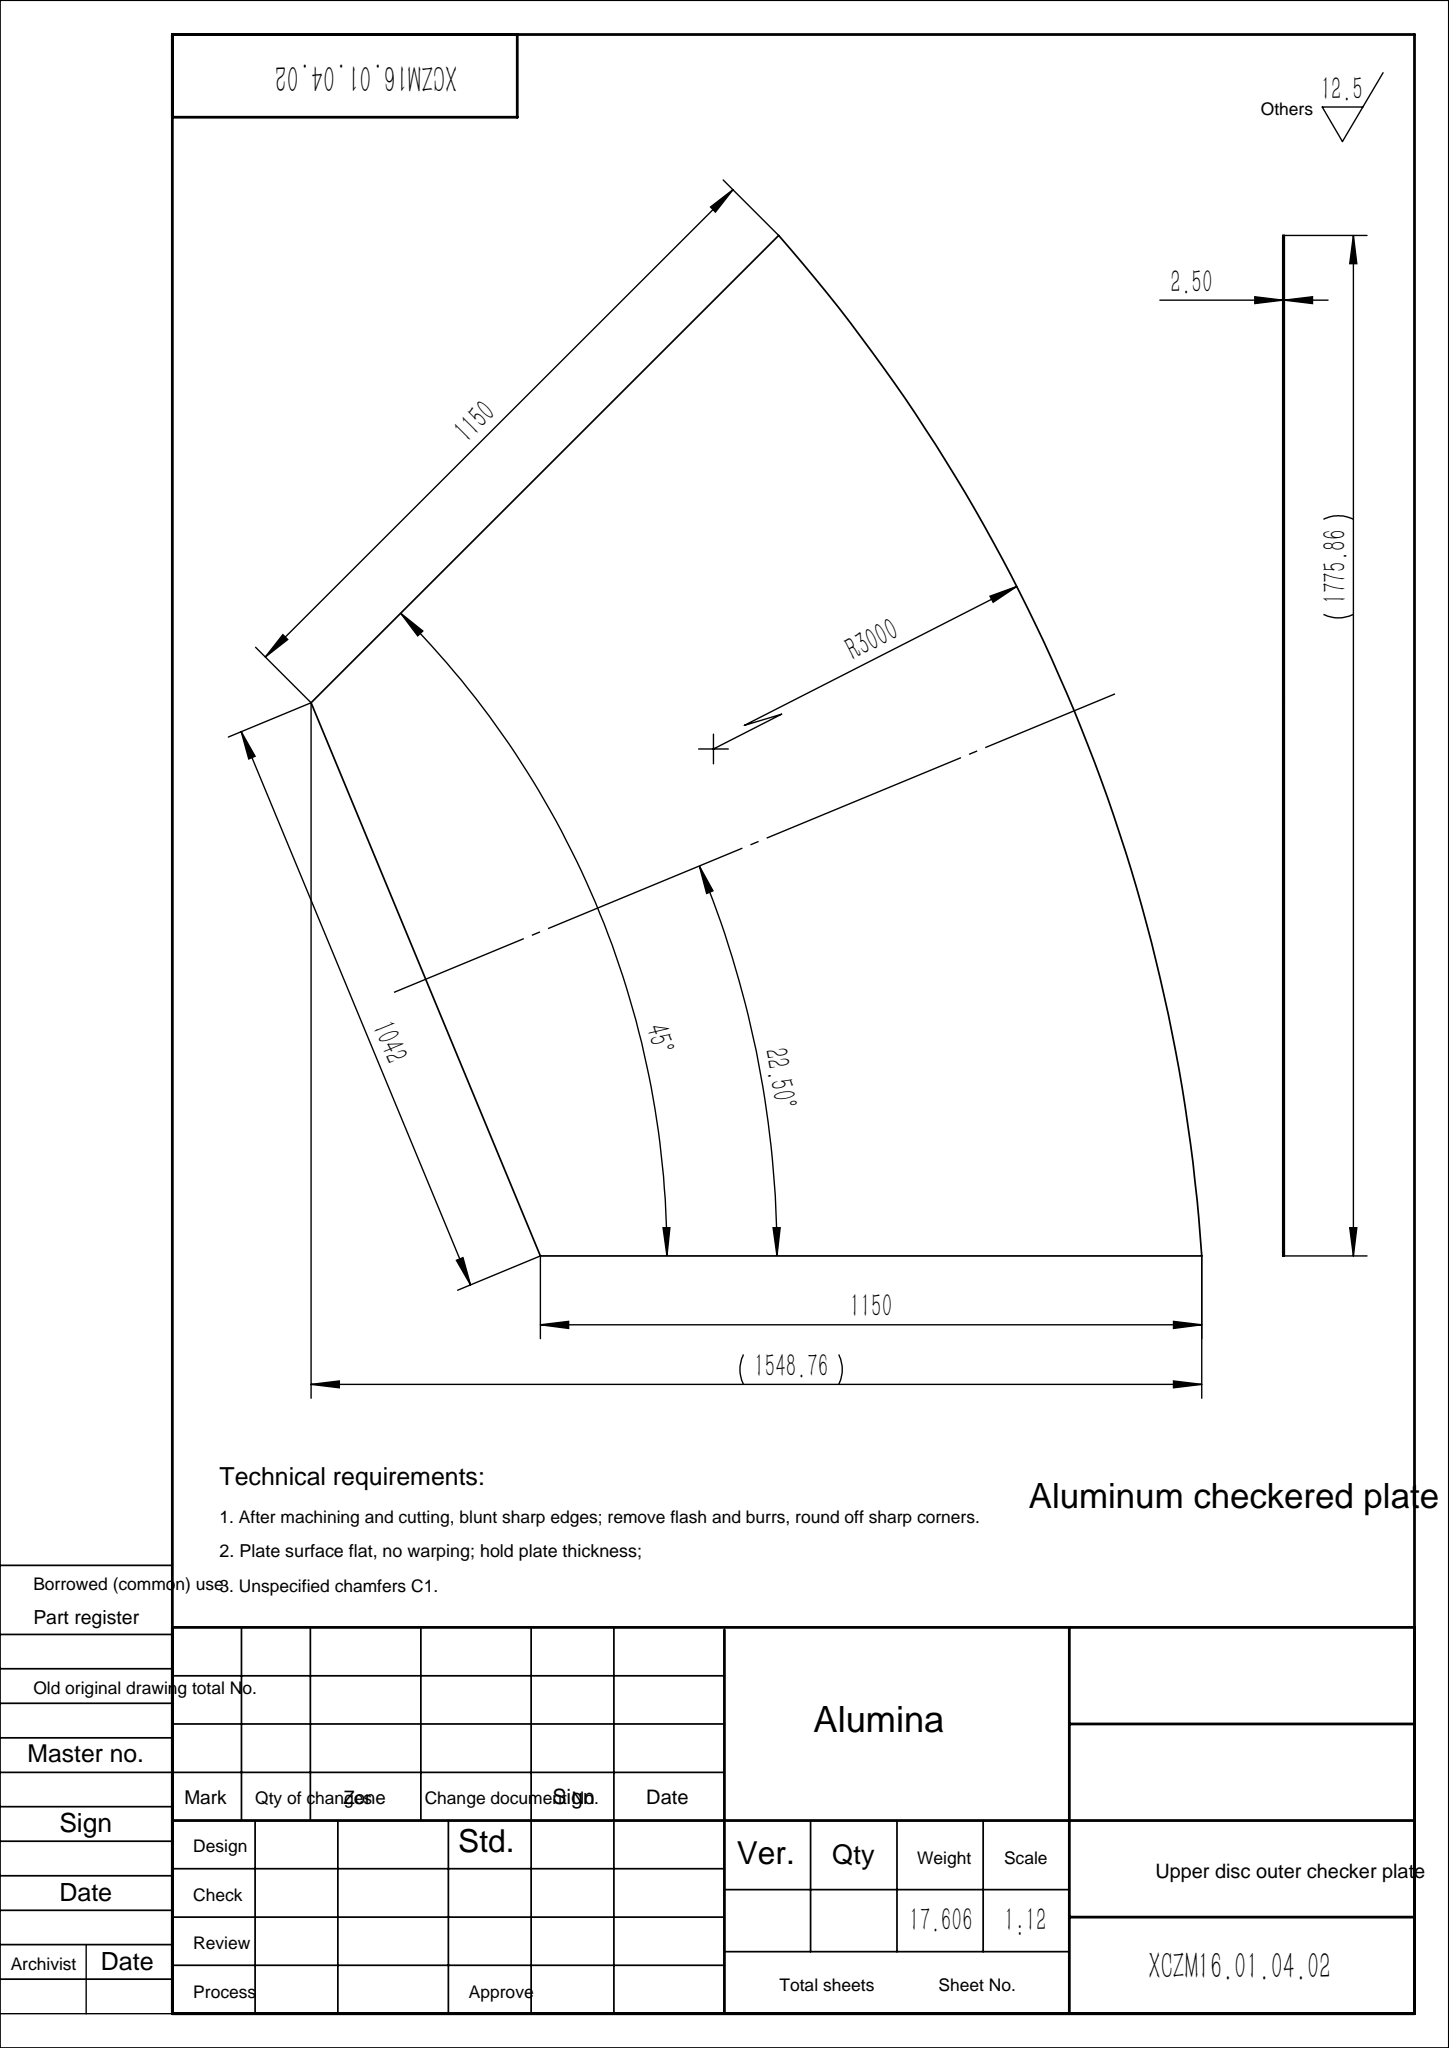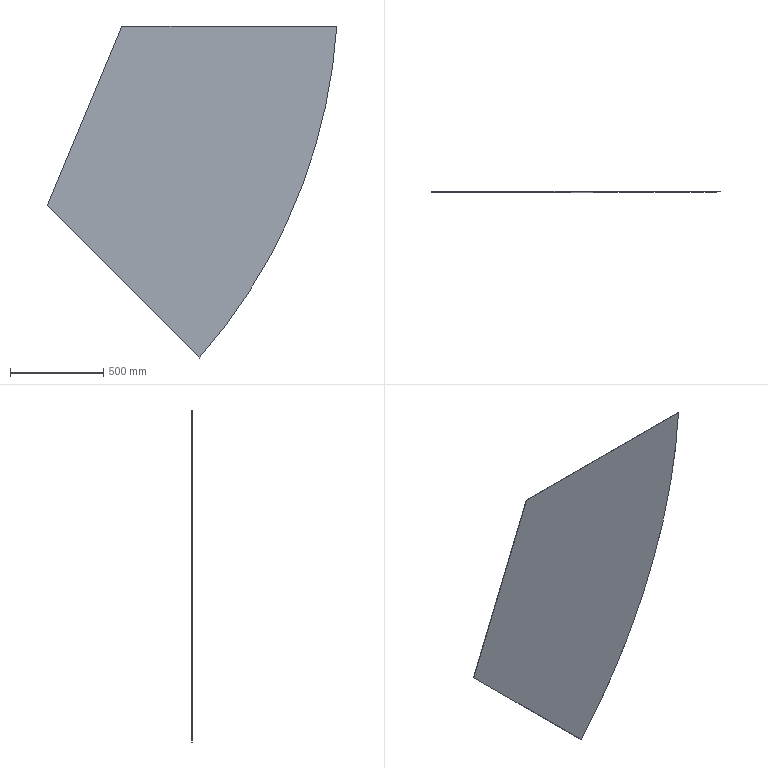Part | SolidWorks | features Extrusion 1 | 1 solid | 6 faces | box 1549 x 2.5 x 1776 mm | volume 4445918 mm3 | plane 5 | cylinder 1 | commonest cylinder face diameters 6000 x1
STEP:
#1=CARTESIAN_POINT('',(0.,0.,0.));
#2=VERTEX_POINT('',#1);
#3=CARTESIAN_POINT('',(1150.,0.,0.));
#4=VERTEX_POINT('',#3);
#5=CARTESIAN_POINT('',(0.,0.,0.));
#6=DIRECTION('',(1.,0.,0.));
#7=VECTOR('',#6,1000.);
#8=LINE('',#5,#7);
#9=EDGE_CURVE('',#2,#4,#8,.T.);
#10=ORIENTED_EDGE('',*,*,#9,.T.);
#11=CARTESIAN_POINT('',(1150.,2.5,0.));
#12=VERTEX_POINT('',#11);
#13=CARTESIAN_POINT('',(1150.,2.5,0.));
#14=DIRECTION('',(0.,-1.,0.));
#15=VECTOR('',#14,1000.);
#16=LINE('',#13,#15);
#17=EDGE_CURVE('',#12,#4,#16,.T.);
#18=ORIENTED_EDGE('',*,*,#17,.F.);
#19=CARTESIAN_POINT('',(0.,2.5,0.));
#20=VERTEX_POINT('',#19);
#21=CARTESIAN_POINT('',(0.,2.5,0.));
#22=DIRECTION('',(1.,0.,0.));
#23=VECTOR('',#22,1000.);
#24=LINE('',#21,#23);
#25=EDGE_CURVE('',#20,#12,#24,.T.);
#26=ORIENTED_EDGE('',*,*,#25,.F.);
#27=CARTESIAN_POINT('',(0.,2.5,0.));
#28=DIRECTION('',(0.,-1.,0.));
#29=VECTOR('',#28,1000.);
#30=LINE('',#27,#29);
#31=EDGE_CURVE('',#20,#2,#30,.T.);
#32=ORIENTED_EDGE('',*,*,#31,.T.);
#33=EDGE_LOOP('',(#10,#18,#26,#32));
#34=FACE_OUTER_BOUND('',#33,.T.);
#35=CARTESIAN_POINT('',(0.,2.5,0.));
#36=DIRECTION('',(0.,0.,-1.));
#37=DIRECTION('',(-1.,0.,0.));
#38=AXIS2_PLACEMENT_3D('',#35,#36,#37);
#39=PLANE('',#38);
#40=ADVANCED_FACE('',(#34),#39,.F.);
#41=CARTESIAN_POINT('',(414.417,0.,-1775.855));
#42=VERTEX_POINT('',#41);
#43=CARTESIAN_POINT('',(-1843.352,0.,199.615));
#44=DIRECTION('',(0.,1.,0.));
#45=DIRECTION('',(0.,0.,1.));
#46=AXIS2_PLACEMENT_3D('',#43,#44,#45);
#47=CIRCLE('',#46,3000.);
#48=EDGE_CURVE('',#4,#42,#47,.T.);
#49=ORIENTED_EDGE('',*,*,#48,.T.);
#50=CARTESIAN_POINT('',(414.417,2.5,-1775.855));
#51=VERTEX_POINT('',#50);
#52=CARTESIAN_POINT('',(414.417,2.5,-1775.855));
#53=DIRECTION('',(0.,-1.,0.));
#54=VECTOR('',#53,1000.);
#55=LINE('',#52,#54);
#56=EDGE_CURVE('',#51,#42,#55,.T.);
#57=ORIENTED_EDGE('',*,*,#56,.F.);
#58=CARTESIAN_POINT('',(-1843.352,2.5,199.615));
#59=DIRECTION('',(0.,1.,0.));
#60=DIRECTION('',(0.,0.,1.));
#61=AXIS2_PLACEMENT_3D('',#58,#59,#60);
#62=CIRCLE('',#61,3000.);
#63=EDGE_CURVE('',#12,#51,#62,.T.);
#64=ORIENTED_EDGE('',*,*,#63,.F.);
#65=ORIENTED_EDGE('',*,*,#17,.T.);
#66=EDGE_LOOP('',(#49,#57,#64,#65));
#67=FACE_OUTER_BOUND('',#66,.T.);
#68=CARTESIAN_POINT('',(-1843.352,2.5,199.615));
#69=DIRECTION('',(0.,-1.,0.));
#70=DIRECTION('',(0.,0.,-1.));
#71=AXIS2_PLACEMENT_3D('',#68,#69,#70);
#72=CYLINDRICAL_SURFACE('',#71,3000.);
#73=ADVANCED_FACE('',(#67),#72,.T.);
#74=CARTESIAN_POINT('',(-398.756,0.,-962.682));
#75=VERTEX_POINT('',#74);
#76=CARTESIAN_POINT('',(414.417,0.,-1775.855));
#77=DIRECTION('',(-0.7071,0.,0.7071));
#78=VECTOR('',#77,1000.);
#79=LINE('',#76,#78);
#80=EDGE_CURVE('',#42,#75,#79,.T.);
#81=ORIENTED_EDGE('',*,*,#80,.T.);
#82=CARTESIAN_POINT('',(-398.756,2.5,-962.682));
#83=VERTEX_POINT('',#82);
#84=CARTESIAN_POINT('',(-398.756,2.5,-962.682));
#85=DIRECTION('',(0.,-1.,0.));
#86=VECTOR('',#85,1000.);
#87=LINE('',#84,#86);
#88=EDGE_CURVE('',#83,#75,#87,.T.);
#89=ORIENTED_EDGE('',*,*,#88,.F.);
#90=CARTESIAN_POINT('',(414.417,2.5,-1775.855));
#91=DIRECTION('',(-0.7071,0.,0.7071));
#92=VECTOR('',#91,1000.);
#93=LINE('',#90,#92);
#94=EDGE_CURVE('',#51,#83,#93,.T.);
#95=ORIENTED_EDGE('',*,*,#94,.F.);
#96=ORIENTED_EDGE('',*,*,#56,.T.);
#97=EDGE_LOOP('',(#81,#89,#95,#96));
#98=FACE_OUTER_BOUND('',#97,.T.);
#99=CARTESIAN_POINT('',(414.417,2.5,-1775.855));
#100=DIRECTION('',(0.7071,0.,0.7071));
#101=DIRECTION('',(0.7071,0.,-0.7071));
#102=AXIS2_PLACEMENT_3D('',#99,#100,#101);
#103=PLANE('',#102);
#104=ADVANCED_FACE('',(#98),#103,.F.);
#105=CARTESIAN_POINT('',(0.,0.,0.));
#106=DIRECTION('',(0.3827,0.,0.9239));
#107=VECTOR('',#106,1000.);
#108=LINE('',#105,#107);
#109=EDGE_CURVE('',#75,#2,#108,.T.);
#110=ORIENTED_EDGE('',*,*,#109,.T.);
#111=ORIENTED_EDGE('',*,*,#31,.F.);
#112=CARTESIAN_POINT('',(0.,2.5,0.));
#113=DIRECTION('',(0.3827,0.,0.9239));
#114=VECTOR('',#113,1000.);
#115=LINE('',#112,#114);
#116=EDGE_CURVE('',#83,#20,#115,.T.);
#117=ORIENTED_EDGE('',*,*,#116,.F.);
#118=ORIENTED_EDGE('',*,*,#88,.T.);
#119=EDGE_LOOP('',(#110,#111,#117,#118));
#120=FACE_OUTER_BOUND('',#119,.T.);
#121=CARTESIAN_POINT('',(0.,2.5,0.));
#122=DIRECTION('',(0.9239,0.,-0.3827));
#123=DIRECTION('',(-0.3827,0.,-0.9239));
#124=AXIS2_PLACEMENT_3D('',#121,#122,#123);
#125=PLANE('',#124);
#126=ADVANCED_FACE('',(#120),#125,.F.);
#127=ORIENTED_EDGE('',*,*,#25,.T.);
#128=ORIENTED_EDGE('',*,*,#63,.T.);
#129=ORIENTED_EDGE('',*,*,#94,.T.);
#130=ORIENTED_EDGE('',*,*,#116,.T.);
#131=EDGE_LOOP('',(#127,#128,#129,#130));
#132=FACE_OUTER_BOUND('',#131,.T.);
#133=CARTESIAN_POINT('',(-1843.352,2.5,199.615));
#134=DIRECTION('',(0.,1.,0.));
#135=DIRECTION('',(0.,0.,1.));
#136=AXIS2_PLACEMENT_3D('',#133,#134,#135);
#137=PLANE('',#136);
#138=ADVANCED_FACE('',(#132),#137,.T.);
#139=ORIENTED_EDGE('',*,*,#9,.F.);
#140=ORIENTED_EDGE('',*,*,#109,.F.);
#141=ORIENTED_EDGE('',*,*,#80,.F.);
#142=ORIENTED_EDGE('',*,*,#48,.F.);
#143=EDGE_LOOP('',(#139,#140,#141,#142));
#144=FACE_OUTER_BOUND('',#143,.T.);
#145=CARTESIAN_POINT('',(-1843.352,0.,199.615));
#146=DIRECTION('',(0.,1.,0.));
#147=DIRECTION('',(0.,0.,1.));
#148=AXIS2_PLACEMENT_3D('',#145,#146,#147);
#149=PLANE('',#148);
#150=ADVANCED_FACE('',(#144),#149,.F.);
#151=CLOSED_SHELL('',(#40,#73,#104,#126,#138,#150));
#152=MANIFOLD_SOLID_BREP('',#151);
#153=CARTESIAN_POINT('',(0.,0.,0.));
#154=DIRECTION('',(0.,0.,1.));
#155=DIRECTION('',(1.,0.,0.));
#156=AXIS2_PLACEMENT_3D('',#153,#154,#155);
#157=(LENGTH_UNIT()NAMED_UNIT(*)SI_UNIT(.MILLI.,.METRE.));
#158=UNCERTAINTY_MEASURE_WITH_UNIT(LENGTH_MEASURE(0.00001),#157,'','');
#159=(NAMED_UNIT(*)PLANE_ANGLE_UNIT()SI_UNIT($,.RADIAN.));
#160=(NAMED_UNIT(*)SI_UNIT($,.STERADIAN.)SOLID_ANGLE_UNIT());
#161=(GEOMETRIC_REPRESENTATION_CONTEXT(3)GLOBAL_UNCERTAINTY_ASSIGNED_CONTEXT((#158))GLOBAL_UNIT_ASSIGNED_CONTEXT((#157,#159,#160))REPRESENTATION_CONTEXT('',''));
#162=ADVANCED_BREP_SHAPE_REPRESENTATION('',(#152,#156),#161);